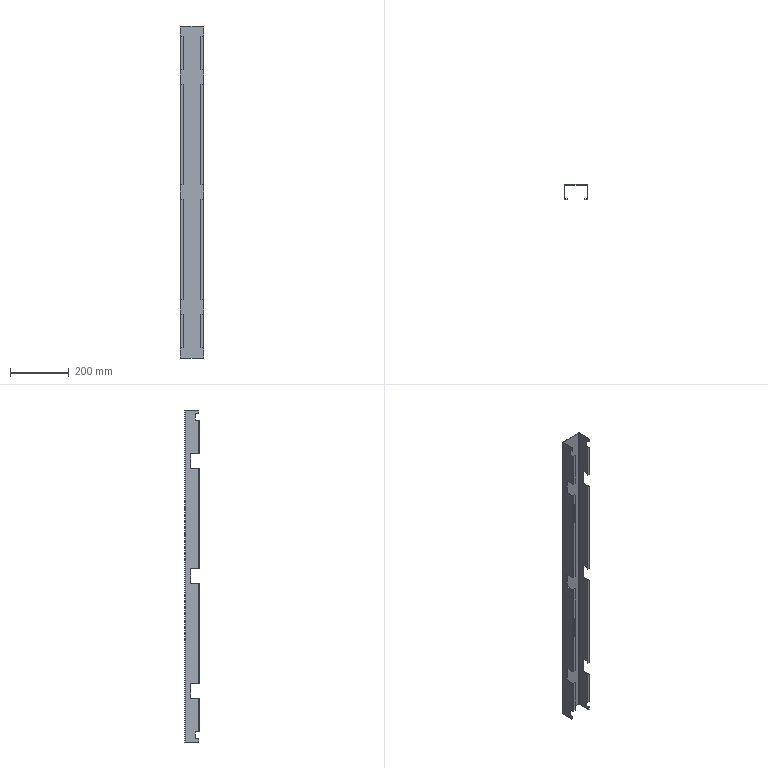Part | SolidWorks | features ICE 3, Chamfer 1, FlatPattern 1, SMBaseFlange 1, SheetMetal 1 | 1 solid | 130 faces | box 80 x 51 x 1130 mm | volume 308482 mm3 | plane 110 | cylinder 20 | commonest cylinder face diameters 0.4 x10 3.4 x10